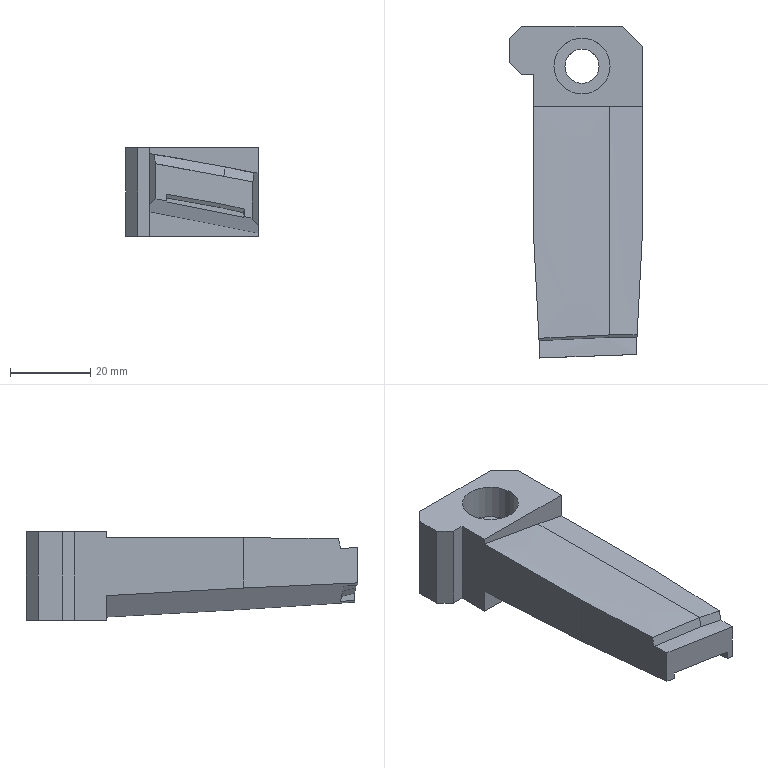Part | STEP file | P011002S001-001 | 1 solid | 29 faces | box 33 x 82.885 x 22 mm | volume 32044 mm3 | plane 20 | spline 4 | other 3 | cylinder 2 | commonest cylinder face diameters 8.5 x1 14 x1